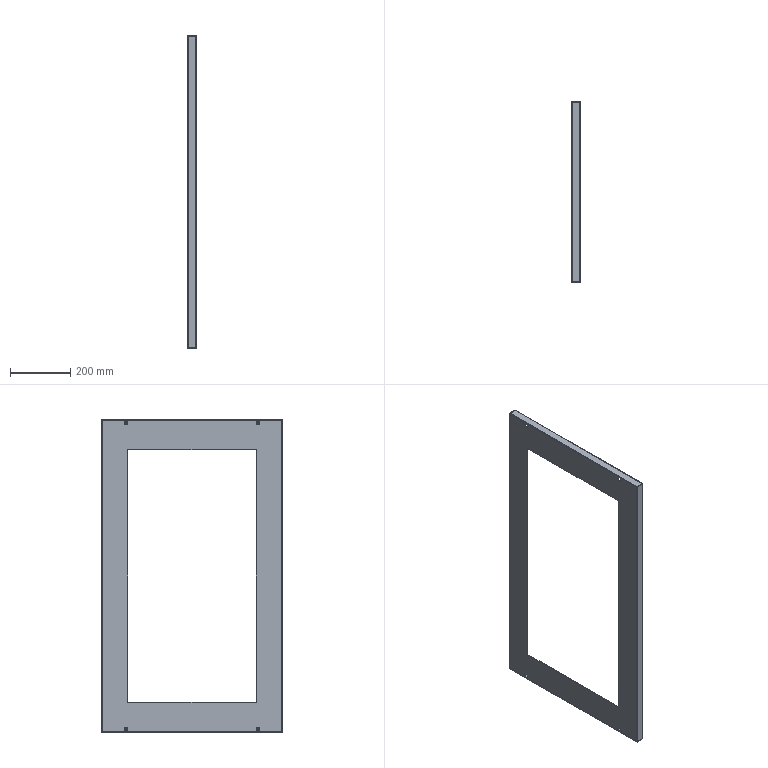Part | STEP file | Left Side Panel | 1 solid | 114 faces | box 28.5 x 597 x 1036 mm | volume 608718 mm3 | plane 66 | cylinder 32 | spline 16 | commonest cylinder face diameters 1 x8 4 x8 7 x8 13 x8